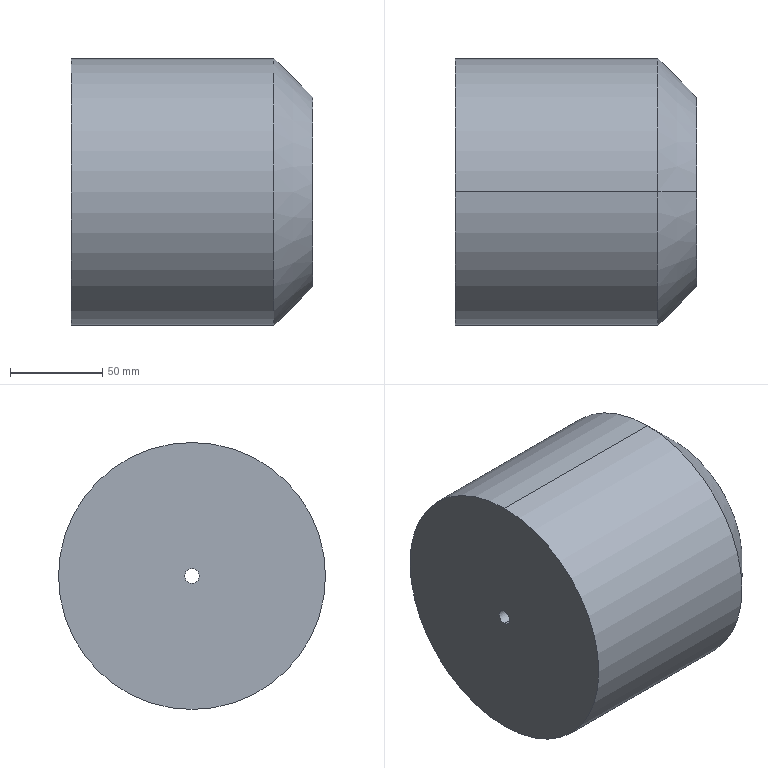Part | SolidWorks | features BaseBody 1 | 1 solid | 8 faces | box 131 x 145 x 145 mm | volume 2065871 mm3 | cylinder 4 | cone 2 | plane 2 | commonest cylinder face diameters 8 x2 145 x2
STEP:
#1=CARTESIAN_POINT('',(339.,0.,-82.587));
#2=VERTEX_POINT('',#1);
#3=CARTESIAN_POINT('',(339.,0.,62.413));
#4=VERTEX_POINT('',#3);
#5=CARTESIAN_POINT('',(339.,0.,-10.087));
#6=DIRECTION('',(1.,0.,0.));
#7=DIRECTION('',(0.,0.,-1.));
#8=AXIS2_PLACEMENT_3D('',#5,#6,#7);
#9=CIRCLE('',#8,72.5);
#10=EDGE_CURVE('',#2,#4,#9,.T.);
#11=ORIENTED_EDGE('',*,*,#10,.T.);
#12=CARTESIAN_POINT('',(449.,0.,62.413));
#13=VERTEX_POINT('',#12);
#14=CARTESIAN_POINT('',(394.,0.,62.413));
#15=DIRECTION('',(1.,0.,0.));
#16=VECTOR('',#15,1000.);
#17=LINE('',#14,#16);
#18=EDGE_CURVE('',#4,#13,#17,.T.);
#19=ORIENTED_EDGE('',*,*,#18,.T.);
#20=CARTESIAN_POINT('',(449.,0.,-82.587));
#21=VERTEX_POINT('',#20);
#22=CARTESIAN_POINT('',(449.,0.,-10.087));
#23=DIRECTION('',(-1.,0.,0.));
#24=DIRECTION('',(0.,0.,-1.));
#25=AXIS2_PLACEMENT_3D('',#22,#23,#24);
#26=CIRCLE('',#25,72.5);
#27=EDGE_CURVE('',#13,#21,#26,.T.);
#28=ORIENTED_EDGE('',*,*,#27,.T.);
#29=CARTESIAN_POINT('',(394.,0.,-82.587));
#30=DIRECTION('',(1.,0.,0.));
#31=VECTOR('',#30,1000.);
#32=LINE('',#29,#31);
#33=EDGE_CURVE('',#2,#21,#32,.T.);
#34=ORIENTED_EDGE('',*,*,#33,.F.);
#35=EDGE_LOOP('',(#11,#19,#28,#34));
#36=FACE_OUTER_BOUND('',#35,.T.);
#37=CARTESIAN_POINT('',(394.,0.,-10.087));
#38=DIRECTION('',(1.,0.,0.));
#39=DIRECTION('',(0.,0.,-1.));
#40=AXIS2_PLACEMENT_3D('',#37,#38,#39);
#41=CYLINDRICAL_SURFACE('',#40,72.5);
#42=ADVANCED_FACE('',(#36),#41,.T.);
#43=CARTESIAN_POINT('',(470.,0.,41.413));
#44=VERTEX_POINT('',#43);
#45=CARTESIAN_POINT('',(470.,0.,-61.587));
#46=VERTEX_POINT('',#45);
#47=CARTESIAN_POINT('',(470.,0.,-10.087));
#48=DIRECTION('',(-1.,0.,0.));
#49=DIRECTION('',(0.,0.,1.));
#50=AXIS2_PLACEMENT_3D('',#47,#48,#49);
#51=CIRCLE('',#50,51.5);
#52=EDGE_CURVE('',#44,#46,#51,.T.);
#53=ORIENTED_EDGE('',*,*,#52,.T.);
#54=CARTESIAN_POINT('',(449.,0.,-82.587));
#55=DIRECTION('',(-0.7071,0.,-0.7071));
#56=VECTOR('',#55,1000.);
#57=LINE('',#54,#56);
#58=EDGE_CURVE('',#46,#21,#57,.T.);
#59=ORIENTED_EDGE('',*,*,#58,.T.);
#60=ORIENTED_EDGE('',*,*,#27,.F.);
#61=CARTESIAN_POINT('',(449.,0.,62.413));
#62=DIRECTION('',(-0.7071,0.,0.7071));
#63=VECTOR('',#62,1000.);
#64=LINE('',#61,#63);
#65=EDGE_CURVE('',#44,#13,#64,.T.);
#66=ORIENTED_EDGE('',*,*,#65,.F.);
#67=EDGE_LOOP('',(#53,#59,#60,#66));
#68=FACE_OUTER_BOUND('',#67,.T.);
#69=CARTESIAN_POINT('',(449.,0.,-10.087));
#70=DIRECTION('',(-1.,0.,0.));
#71=DIRECTION('',(0.,0.,1.));
#72=AXIS2_PLACEMENT_3D('',#69,#70,#71);
#73=CONICAL_SURFACE('',#72,72.5,0.7854);
#74=ADVANCED_FACE('',(#68),#73,.T.);
#75=CARTESIAN_POINT('',(339.,0.,-6.087));
#76=VERTEX_POINT('',#75);
#77=CARTESIAN_POINT('',(339.,0.,-14.087));
#78=VERTEX_POINT('',#77);
#79=CARTESIAN_POINT('',(339.,0.,-10.087));
#80=DIRECTION('',(1.,0.,0.));
#81=DIRECTION('',(0.,0.,-1.));
#82=AXIS2_PLACEMENT_3D('',#79,#80,#81);
#83=CIRCLE('',#82,4.);
#84=EDGE_CURVE('',#76,#78,#83,.T.);
#85=ORIENTED_EDGE('',*,*,#84,.F.);
#86=CARTESIAN_POINT('',(470.,0.,-6.087));
#87=VERTEX_POINT('',#86);
#88=CARTESIAN_POINT('',(404.5,0.,-6.087));
#89=DIRECTION('',(1.,0.,0.));
#90=VECTOR('',#89,1000.);
#91=LINE('',#88,#90);
#92=EDGE_CURVE('',#76,#87,#91,.T.);
#93=ORIENTED_EDGE('',*,*,#92,.T.);
#94=CARTESIAN_POINT('',(470.,0.,-14.087));
#95=VERTEX_POINT('',#94);
#96=CARTESIAN_POINT('',(470.,0.,-10.087));
#97=DIRECTION('',(-1.,0.,0.));
#98=DIRECTION('',(0.,0.,-1.));
#99=AXIS2_PLACEMENT_3D('',#96,#97,#98);
#100=CIRCLE('',#99,4.);
#101=EDGE_CURVE('',#95,#87,#100,.T.);
#102=ORIENTED_EDGE('',*,*,#101,.F.);
#103=CARTESIAN_POINT('',(404.5,0.,-14.087));
#104=DIRECTION('',(1.,0.,0.));
#105=VECTOR('',#104,1000.);
#106=LINE('',#103,#105);
#107=EDGE_CURVE('',#78,#95,#106,.T.);
#108=ORIENTED_EDGE('',*,*,#107,.F.);
#109=EDGE_LOOP('',(#85,#93,#102,#108));
#110=FACE_OUTER_BOUND('',#109,.T.);
#111=CARTESIAN_POINT('',(404.5,0.,-10.087));
#112=DIRECTION('',(1.,0.,0.));
#113=DIRECTION('',(0.,0.,-1.));
#114=AXIS2_PLACEMENT_3D('',#111,#112,#113);
#115=CYLINDRICAL_SURFACE('',#114,4.);
#116=ADVANCED_FACE('',(#110),#115,.F.);
#117=ORIENTED_EDGE('',*,*,#18,.F.);
#118=CARTESIAN_POINT('',(339.,0.,-10.087));
#119=DIRECTION('',(1.,0.,0.));
#120=DIRECTION('',(0.,0.,-1.));
#121=AXIS2_PLACEMENT_3D('',#118,#119,#120);
#122=CIRCLE('',#121,72.5);
#123=EDGE_CURVE('',#4,#2,#122,.T.);
#124=ORIENTED_EDGE('',*,*,#123,.T.);
#125=ORIENTED_EDGE('',*,*,#33,.T.);
#126=CARTESIAN_POINT('',(449.,0.,-10.087));
#127=DIRECTION('',(-1.,0.,0.));
#128=DIRECTION('',(0.,0.,-1.));
#129=AXIS2_PLACEMENT_3D('',#126,#127,#128);
#130=CIRCLE('',#129,72.5);
#131=EDGE_CURVE('',#21,#13,#130,.T.);
#132=ORIENTED_EDGE('',*,*,#131,.T.);
#133=EDGE_LOOP('',(#117,#124,#125,#132));
#134=FACE_OUTER_BOUND('',#133,.T.);
#135=CARTESIAN_POINT('',(394.,0.,-10.087));
#136=DIRECTION('',(1.,0.,0.));
#137=DIRECTION('',(0.,0.,-1.));
#138=AXIS2_PLACEMENT_3D('',#135,#136,#137);
#139=CYLINDRICAL_SURFACE('',#138,72.5);
#140=ADVANCED_FACE('',(#134),#139,.T.);
#141=CARTESIAN_POINT('',(339.,0.,-10.087));
#142=DIRECTION('',(1.,0.,0.));
#143=DIRECTION('',(0.,0.,-1.));
#144=AXIS2_PLACEMENT_3D('',#141,#142,#143);
#145=CIRCLE('',#144,4.);
#146=EDGE_CURVE('',#78,#76,#145,.T.);
#147=ORIENTED_EDGE('',*,*,#146,.T.);
#148=ORIENTED_EDGE('',*,*,#84,.T.);
#149=EDGE_LOOP('',(#147,#148));
#150=FACE_BOUND('',#149,.T.);
#151=ORIENTED_EDGE('',*,*,#10,.F.);
#152=ORIENTED_EDGE('',*,*,#123,.F.);
#153=EDGE_LOOP('',(#151,#152));
#154=FACE_OUTER_BOUND('',#153,.T.);
#155=CARTESIAN_POINT('',(339.,0.,-10.087));
#156=DIRECTION('',(-1.,0.,0.));
#157=DIRECTION('',(0.,0.,1.));
#158=AXIS2_PLACEMENT_3D('',#155,#156,#157);
#159=PLANE('',#158);
#160=ADVANCED_FACE('',(#150,#154),#159,.T.);
#161=ORIENTED_EDGE('',*,*,#58,.F.);
#162=CARTESIAN_POINT('',(470.,0.,-10.087));
#163=DIRECTION('',(-1.,0.,0.));
#164=DIRECTION('',(0.,0.,1.));
#165=AXIS2_PLACEMENT_3D('',#162,#163,#164);
#166=CIRCLE('',#165,51.5);
#167=EDGE_CURVE('',#46,#44,#166,.T.);
#168=ORIENTED_EDGE('',*,*,#167,.T.);
#169=ORIENTED_EDGE('',*,*,#65,.T.);
#170=ORIENTED_EDGE('',*,*,#131,.F.);
#171=EDGE_LOOP('',(#161,#168,#169,#170));
#172=FACE_OUTER_BOUND('',#171,.T.);
#173=CARTESIAN_POINT('',(449.,0.,-10.087));
#174=DIRECTION('',(-1.,0.,0.));
#175=DIRECTION('',(0.,0.,1.));
#176=AXIS2_PLACEMENT_3D('',#173,#174,#175);
#177=CONICAL_SURFACE('',#176,72.5,0.7854);
#178=ADVANCED_FACE('',(#172),#177,.T.);
#179=ORIENTED_EDGE('',*,*,#92,.F.);
#180=ORIENTED_EDGE('',*,*,#146,.F.);
#181=ORIENTED_EDGE('',*,*,#107,.T.);
#182=CARTESIAN_POINT('',(470.,0.,-10.087));
#183=DIRECTION('',(-1.,0.,0.));
#184=DIRECTION('',(0.,0.,-1.));
#185=AXIS2_PLACEMENT_3D('',#182,#183,#184);
#186=CIRCLE('',#185,4.);
#187=EDGE_CURVE('',#87,#95,#186,.T.);
#188=ORIENTED_EDGE('',*,*,#187,.F.);
#189=EDGE_LOOP('',(#179,#180,#181,#188));
#190=FACE_OUTER_BOUND('',#189,.T.);
#191=CARTESIAN_POINT('',(404.5,0.,-10.087));
#192=DIRECTION('',(1.,0.,0.));
#193=DIRECTION('',(0.,0.,-1.));
#194=AXIS2_PLACEMENT_3D('',#191,#192,#193);
#195=CYLINDRICAL_SURFACE('',#194,4.);
#196=ADVANCED_FACE('',(#190),#195,.F.);
#197=ORIENTED_EDGE('',*,*,#101,.T.);
#198=ORIENTED_EDGE('',*,*,#187,.T.);
#199=EDGE_LOOP('',(#197,#198));
#200=FACE_BOUND('',#199,.T.);
#201=ORIENTED_EDGE('',*,*,#52,.F.);
#202=ORIENTED_EDGE('',*,*,#167,.F.);
#203=EDGE_LOOP('',(#201,#202));
#204=FACE_OUTER_BOUND('',#203,.T.);
#205=CARTESIAN_POINT('',(470.,0.,-10.087));
#206=DIRECTION('',(-1.,0.,0.));
#207=DIRECTION('',(0.,0.,1.));
#208=AXIS2_PLACEMENT_3D('',#205,#206,#207);
#209=PLANE('',#208);
#210=ADVANCED_FACE('',(#200,#204),#209,.F.);
#211=CLOSED_SHELL('',(#42,#74,#116,#140,#160,#178,#196,#210));
#212=MANIFOLD_SOLID_BREP('',#211);
#213=CARTESIAN_POINT('',(0.,0.,0.));
#214=DIRECTION('',(0.,0.,1.));
#215=DIRECTION('',(1.,0.,0.));
#216=AXIS2_PLACEMENT_3D('',#213,#214,#215);
#217=(LENGTH_UNIT()NAMED_UNIT(*)SI_UNIT(.MILLI.,.METRE.));
#218=UNCERTAINTY_MEASURE_WITH_UNIT(LENGTH_MEASURE(0.00001),#217,'','');
#219=(NAMED_UNIT(*)PLANE_ANGLE_UNIT()SI_UNIT($,.RADIAN.));
#220=(NAMED_UNIT(*)SI_UNIT($,.STERADIAN.)SOLID_ANGLE_UNIT());
#221=(GEOMETRIC_REPRESENTATION_CONTEXT(3)GLOBAL_UNCERTAINTY_ASSIGNED_CONTEXT((#218))GLOBAL_UNIT_ASSIGNED_CONTEXT((#217,#219,#220))REPRESENTATION_CONTEXT('',''));
#222=ADVANCED_BREP_SHAPE_REPRESENTATION('',(#212,#216),#221);